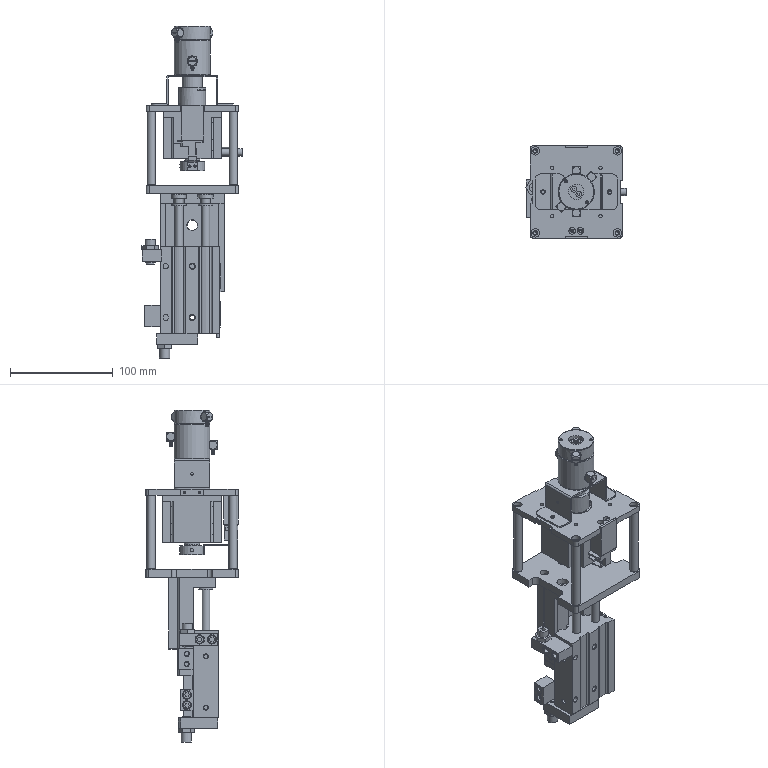Part | NX | 42 solids | 1239 faces | box 97.583 x 90 x 323.8 mm | volume 631883 mm3 | plane 684 | cylinder 389 | cone 125 | spline 41 | commonest cylinder face diameters 10 x29 2.5 x28 8 x24 3.3 x21 4.134 x18 5 x15